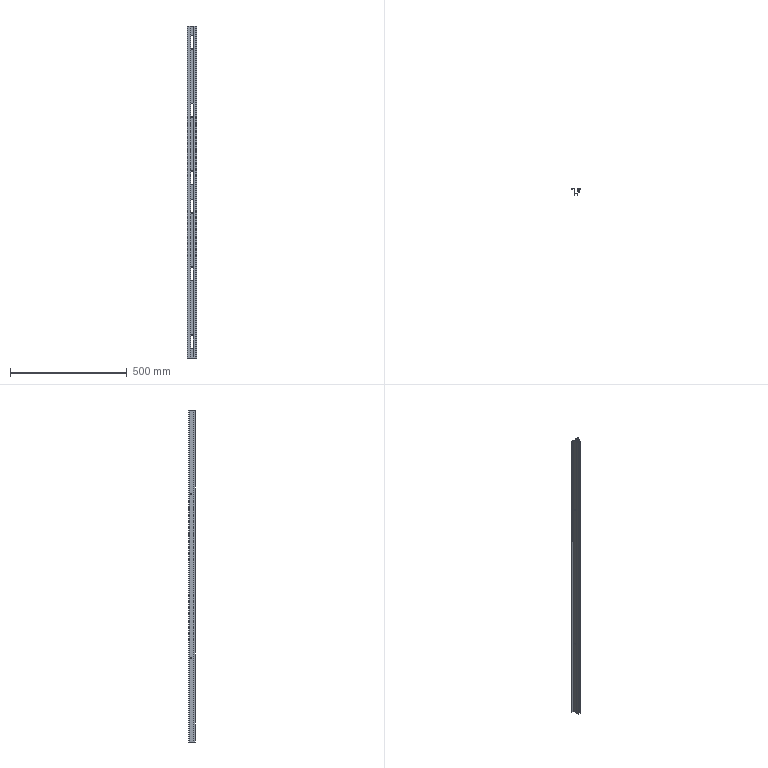Part | 1 solid | 102 faces | box 40 x 29.5 x 1420 mm | volume 266399 mm3 | plane 65 | cylinder 37 | commonest cylinder face diameters 9 x30 2 x5 3 x2